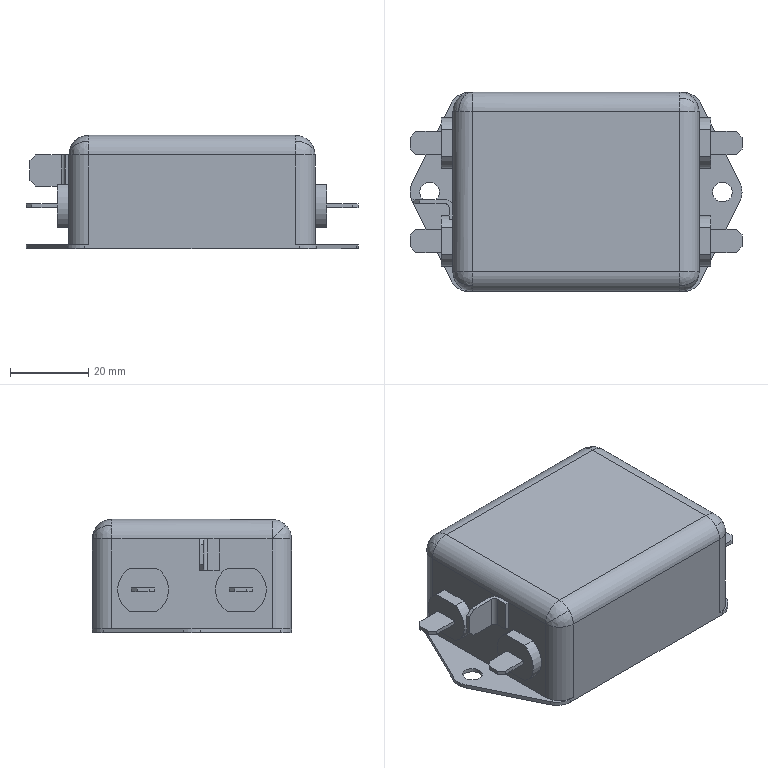Part | STEP file | filter CW4EL2-30A-S | 1 solid | 98 faces | box 85 x 51 x 29 mm | volume 93702 mm3 | plane 61 | cylinder 29 | spline 8 | commonest cylinder face diameters 10 x15 13 x8 5 x4 2 x1 4 x1